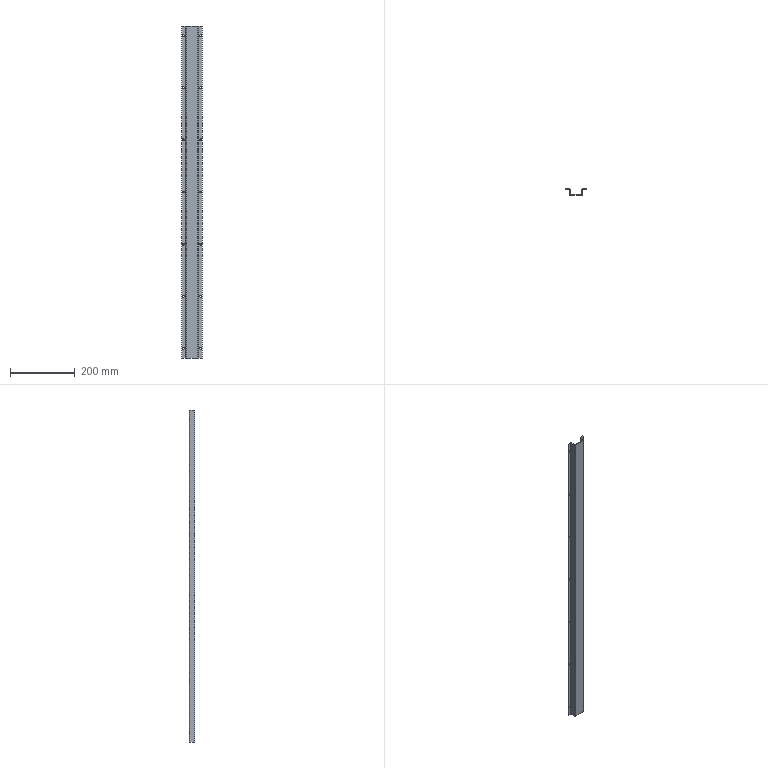Part | NX | features solid 2 | 1 solid | 50 faces | box 64 x 18.5 x 1028 mm | volume 144566 mm3 | cylinder 36 | plane 14 | commonest cylinder face diameters 6 x32 3 x4